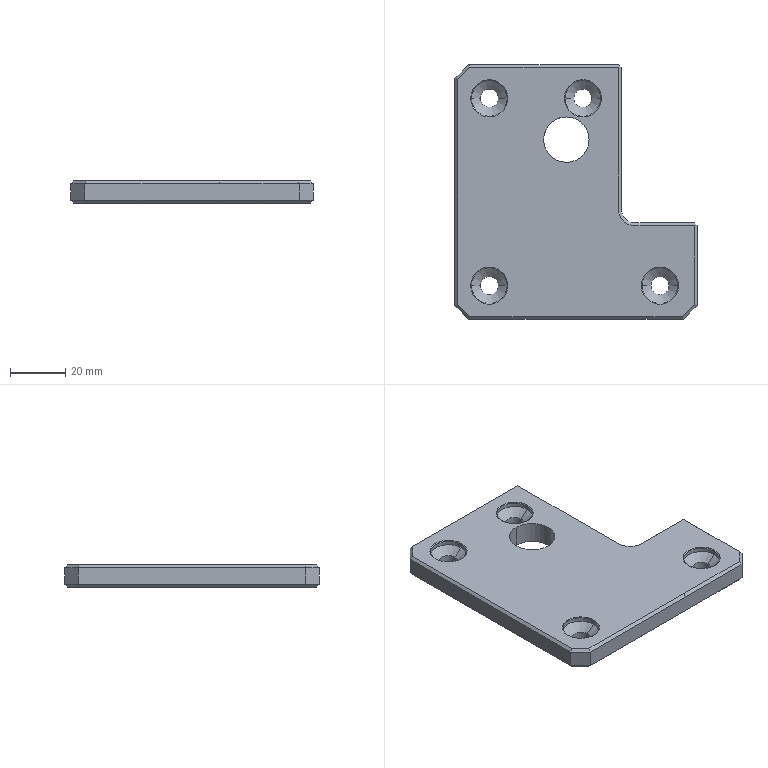Part | Creo | 1 solid | 70 faces | box 88 x 92.5 x 8 mm | volume 47874 mm3 | plane 33 | cylinder 19 | cone 18 | commonest cylinder face diameters 6.6 x8 13 x8 16.5 x2 10 x1